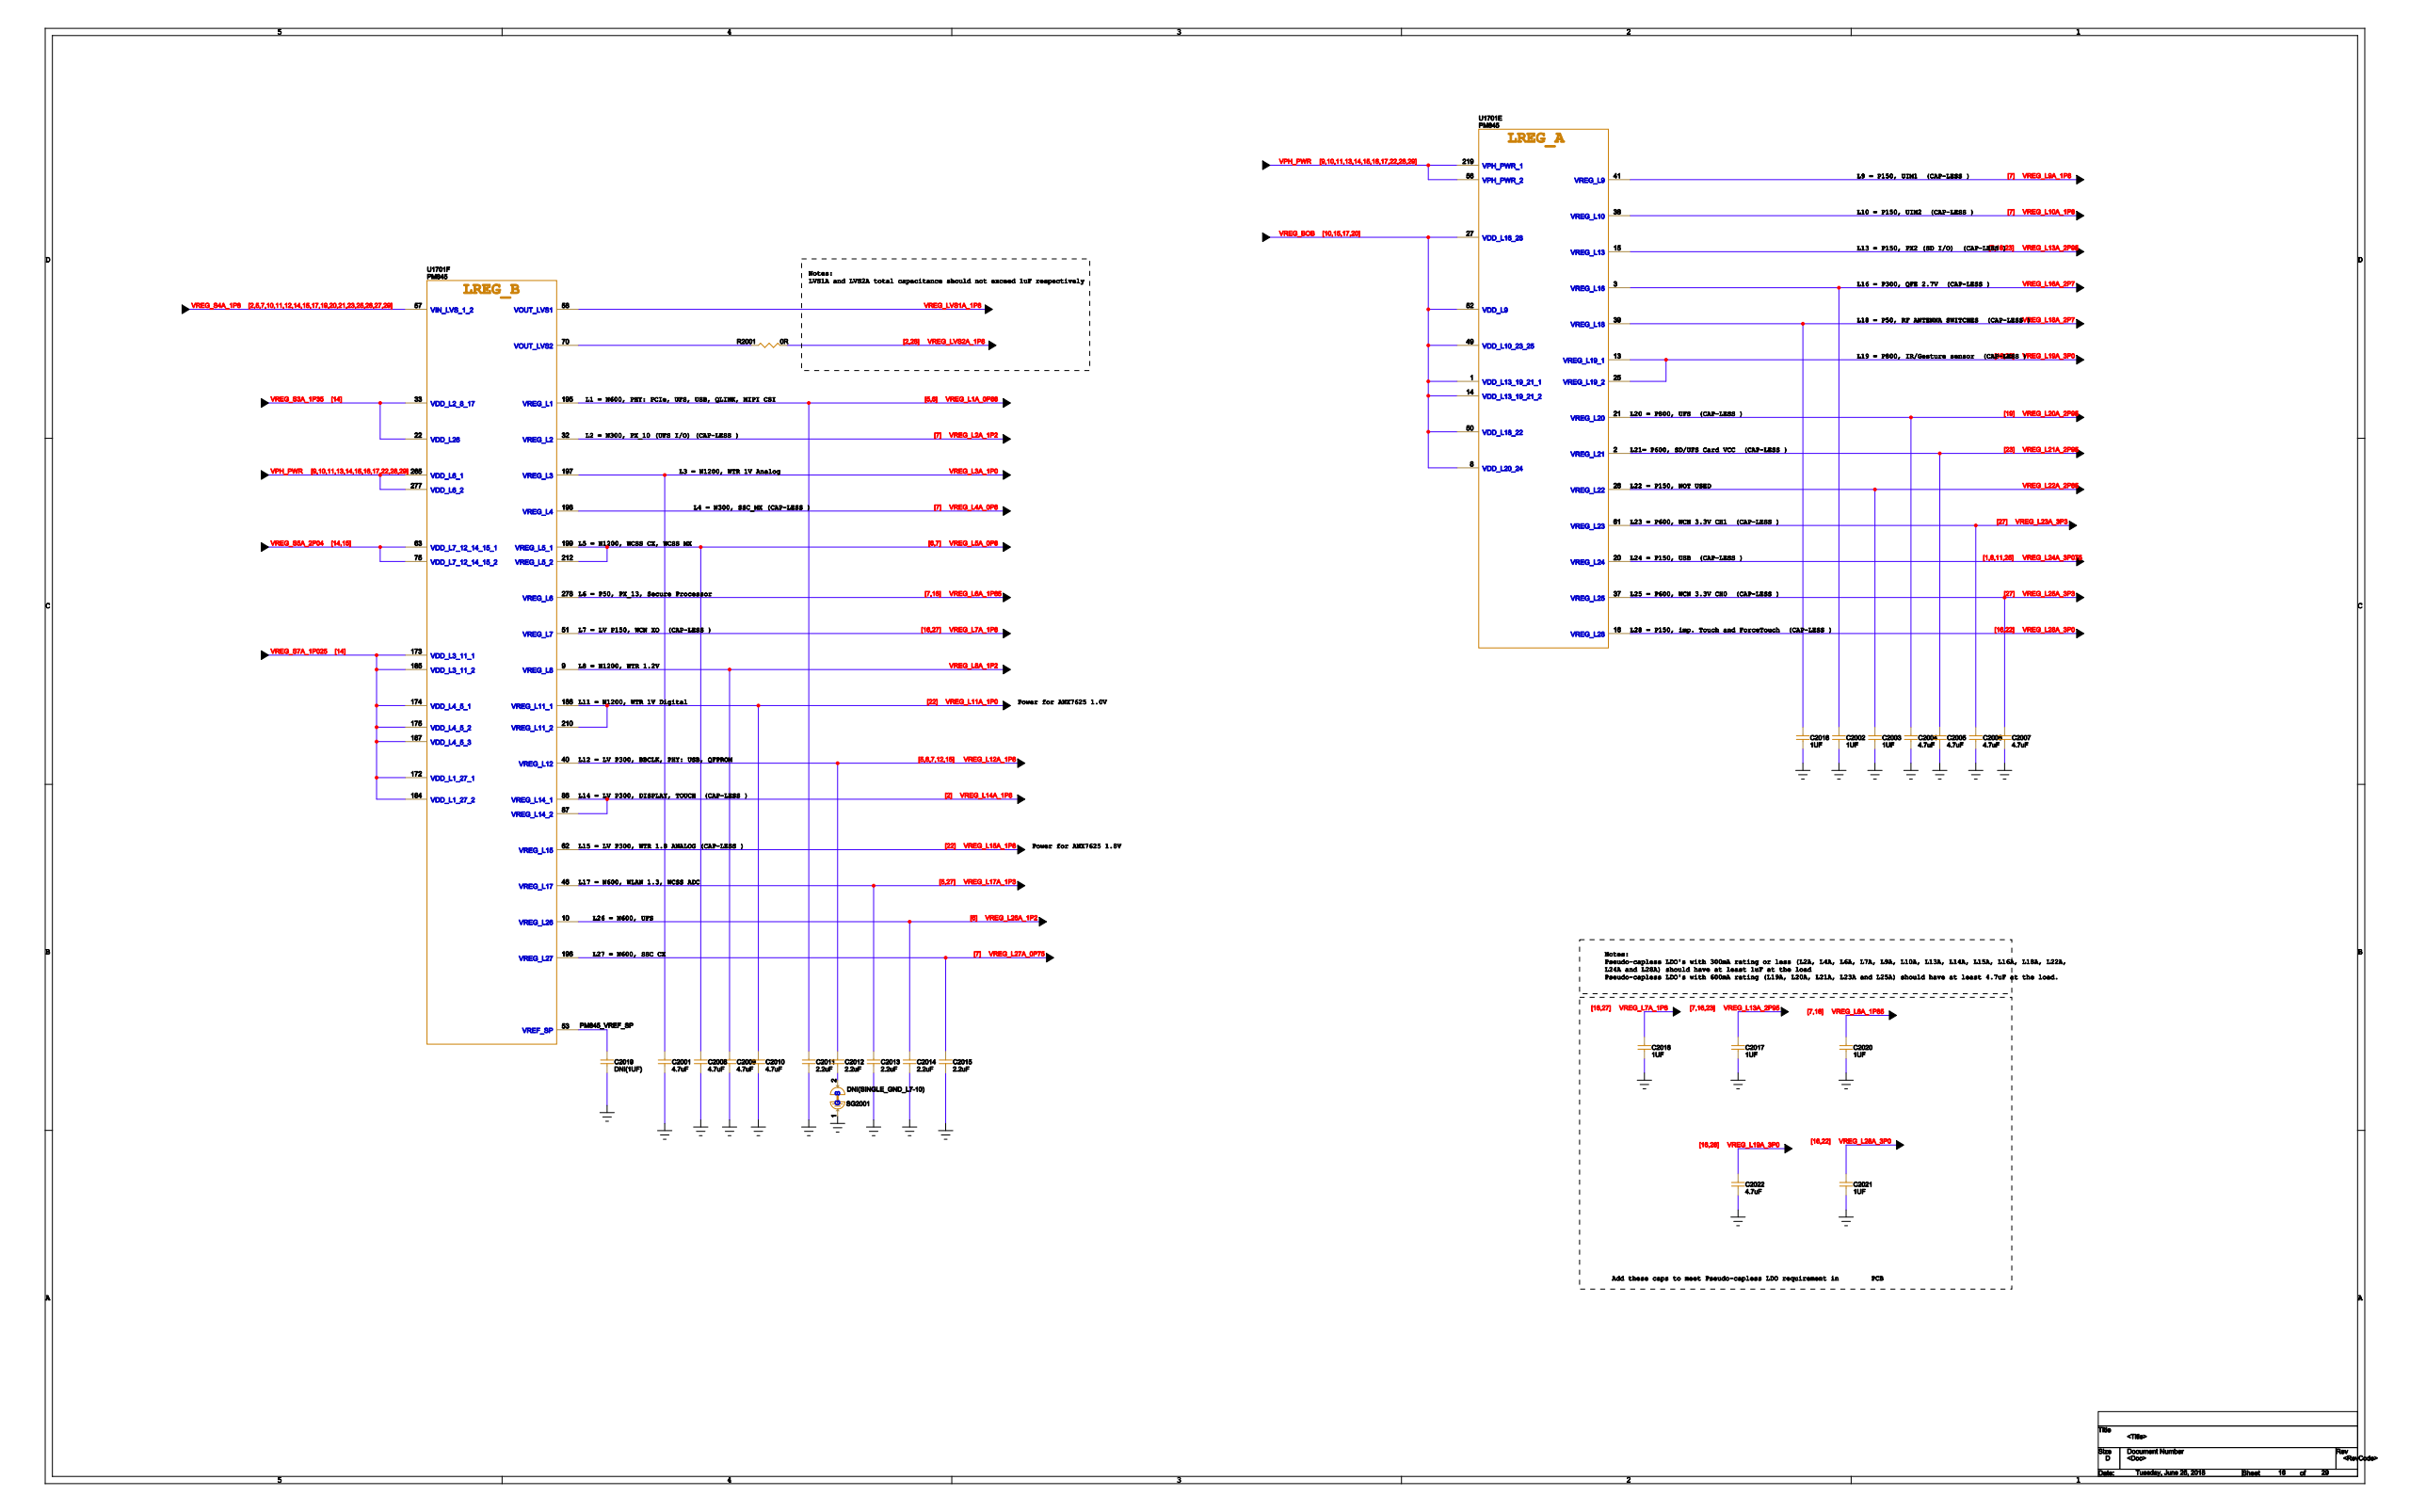Circuit board | Cadence Allegro | 802 parts | 566 nets | one sheet of the schematic
Parts on this sheet (reference | value | footprint):
C2001 | 4.7uF | 0402-BIG
C2002 | 1uF | C0201
C2003 | 1uF | C0201
C2004 | 4.7uF | 0402-BIG
C2005 | 4.7uF | 0402-BIG
C2006 | 4.7uF | 0402-BIG
C2007 | 4.7uF | 0402-BIG
C2008 | 4.7uF | 0402-BIG
C2009 | 4.7uF | 0402-BIG
C2010 | 4.7uF | 0402-BIG
C2011 | 2.2uF | 0402-BIG
C2012 | 2.2uF | 0402-BIG
C2013 | 2.2uF | 0402-BIG
C2014 | 2.2uF | 0402-BIG
C2015 | 2.2uF | 0402-BIG
C2016 | 1uF | C0201
C2017 | 1uF | C0201
C2018 | 1uF | C0201
C2019 | DNI(1UF) | C0201
C2020 | 1uF | C0201
C2021 | 1uF | C0201
C2022 | 4.7uF | 0402-BIG
R2001 | 0R | R0201
SG2001 | DNI(SINGLE_GND_L7-10) | GND_L7-10
U1701 | PM845 | PM8998
Nets of these parts (net: part-pin ...):
GND: C2001-2 C2002-2 C2003-2 C2004-2 C2005-2 C2006-2 C2007-2 C2008-2 C2009-2 C2010-2 C2011-2 C2013-2 C2014-2 C2015-2 C2016-2 C2017-2 C2018-2 C2019-2 C2020-2 C2021-2 C2022-2 SG2001-1 U1701-7
VREG_L25A_3P3: C2007-1 U1701-37
VREG_L24A_3P075: U1701-20
VREG_L20A_2P95: C2004-1 U1701-21
VREG_L28A_3P0: C2021-1 U1701-16
VPH_PWR: U1701-56 U1701-219 U1701-265 U1701-277
VREG_S4A_1P8: U1701-57
VREG_L19A_3P0: C2022-1 U1701-13 U1701-25
VREG_LVS2A_1P8: R2001-2
PM845_VREF_SP: C2019-1 U1701-53
VREG_L7A_1P8: C2016-1 U1701-51
VREG_BOB: U1701-1 U1701-8 U1701-14 U1701-27 U1701-49 U1701-50 U1701-52
N249216: R2001-1 U1701-70
VREG_L6A_1P85: C2020-1 U1701-278
VREG_L13A_2P95: C2017-1 U1701-15
VREG_L16A_2P7: C2002-1 U1701-3
VREG_L22A_2P85: C2003-1 U1701-26
VREG_L18A_2P7: C2018-1 U1701-39
VREG_L21A_2P95: C2005-1 U1701-2
VREG_L17A_1P3: C2013-1 U1701-46
VREG_L1A_0P88: C2011-1 U1701-195
VREG_L12A_1P8: C2012-1 U1701-28 U1701-40
VREG_L26A_1P2: C2014-1 U1701-10
VREG_L5A_0P8: C2008-1 U1701-199 U1701-212
VREG_L9A_1P8: U1701-41
VREG_L10A_1P8: U1701-38
VREG_L2A_1P2: U1701-32
VREG_L27A_0P75: C2015-1 U1701-196
VREG_L4A_0P8: U1701-198
VREG_S3A_1P35: U1701-22 U1701-33
VREG_S5A_2P04: U1701-29 U1701-63 U1701-75
VREG_S7A_1P025: U1701-172 U1701-173 U1701-174 U1701-175 U1701-184 U1701-185 U1701-187
N248212: C2012-2 SG2001-2
VREG_L3A_1P0: C2001-1 U1701-197
VREG_L23A_3P3: C2006-1 U1701-61
VREG_L8A_1P2: C2009-1 U1701-9
VREG_L11A_1P0: C2010-1 U1701-186 U1701-210
VREG_L14A_1P8: U1701-86 U1701-87
VREG_L15A_1P8: U1701-62
VREG_LVS1A_1P8: U1701-58